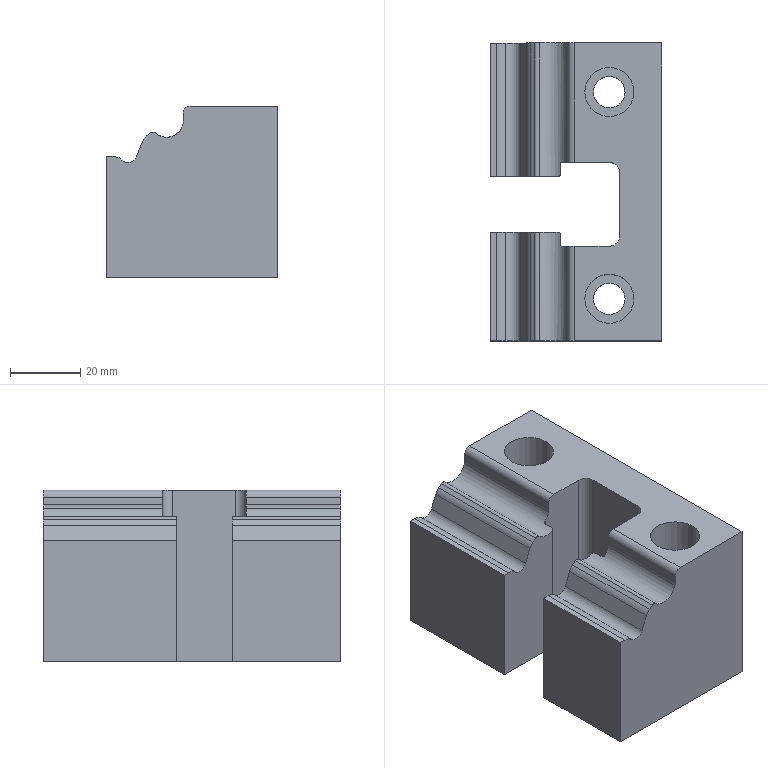Part | 1 solid | 52 faces | box 49 x 85 x 48.948 mm | volume 143293 mm3 | cylinder 28 | plane 24 | commonest cylinder face diameters 1 x4 9 x4 9.5 x4 14 x4 2 x2 4 x2